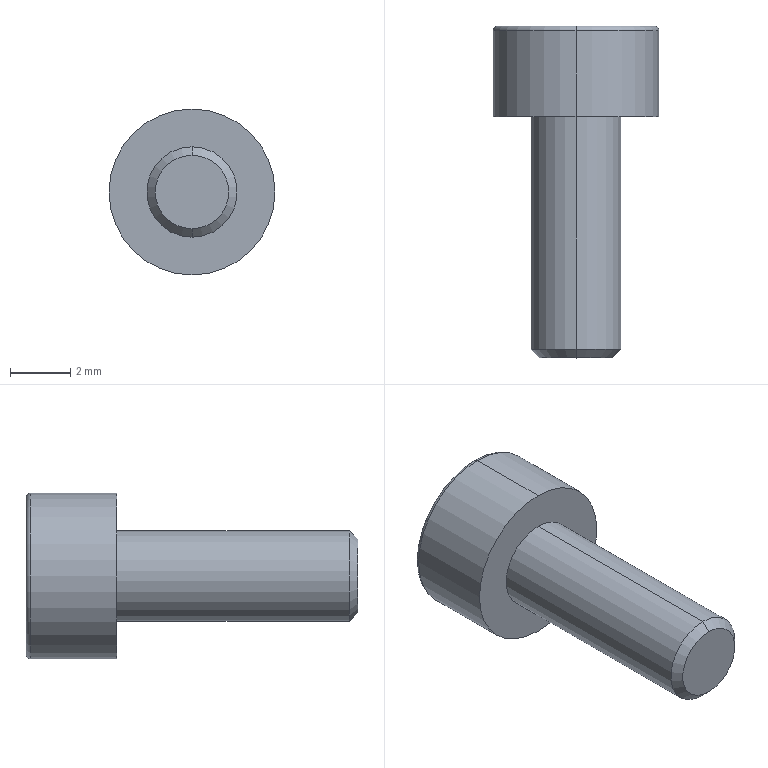Part | SolidWorks | features ICE 2, Chamfer 1, Extrusion 1, Fillet 1, RefAxis 1 | 1 solid | 18 faces | box 5.5 x 11 x 5.5 mm | volume 120.016 mm3 | plane 10 | cylinder 4 | cone 2 | torus 2 | commonest cylinder face diameters 3 x2 5.5 x2
STEP:
#1=CARTESIAN_POINT('',(0.,-8.,-1.22));
#2=VERTEX_POINT('',#1);
#3=CARTESIAN_POINT('',(0.,-8.,1.22));
#4=VERTEX_POINT('',#3);
#5=CARTESIAN_POINT('',(0.,-8.,0.));
#6=DIRECTION('',(0.,-1.,0.));
#7=DIRECTION('',(0.,0.,-1.));
#8=AXIS2_PLACEMENT_3D('',#5,#6,#7);
#9=CIRCLE('',#8,1.22);
#10=EDGE_CURVE('',#2,#4,#9,.T.);
#11=ORIENTED_EDGE('',*,*,#10,.F.);
#12=CARTESIAN_POINT('',(0.,-7.72,-1.5));
#13=VERTEX_POINT('',#12);
#14=CARTESIAN_POINT('',(0.,-8.,-1.22));
#15=DIRECTION('',(0.,0.7071,-0.7071));
#16=VECTOR('',#15,1000.);
#17=LINE('',#14,#16);
#18=EDGE_CURVE('',#2,#13,#17,.T.);
#19=ORIENTED_EDGE('',*,*,#18,.T.);
#20=CARTESIAN_POINT('',(0.,-7.72,1.5));
#21=VERTEX_POINT('',#20);
#22=CARTESIAN_POINT('',(0.,-7.72,0.));
#23=DIRECTION('',(0.,1.,0.));
#24=DIRECTION('',(0.,0.,-1.));
#25=AXIS2_PLACEMENT_3D('',#22,#23,#24);
#26=CIRCLE('',#25,1.5);
#27=EDGE_CURVE('',#21,#13,#26,.T.);
#28=ORIENTED_EDGE('',*,*,#27,.F.);
#29=CARTESIAN_POINT('',(0.,-8.,1.22));
#30=DIRECTION('',(0.,0.7071,0.7071));
#31=VECTOR('',#30,1000.);
#32=LINE('',#29,#31);
#33=EDGE_CURVE('',#4,#21,#32,.T.);
#34=ORIENTED_EDGE('',*,*,#33,.F.);
#35=EDGE_LOOP('',(#11,#19,#28,#34));
#36=FACE_OUTER_BOUND('',#35,.T.);
#37=CARTESIAN_POINT('',(0.,-8.,0.));
#38=DIRECTION('',(0.,1.,0.));
#39=DIRECTION('',(0.,0.,1.));
#40=AXIS2_PLACEMENT_3D('',#37,#38,#39);
#41=CONICAL_SURFACE('',#40,1.22,0.7854);
#42=ADVANCED_FACE('',(#36),#41,.T.);
#43=ORIENTED_EDGE('',*,*,#27,.T.);
#44=CARTESIAN_POINT('',(0.,0.,-1.5));
#45=VERTEX_POINT('',#44);
#46=CARTESIAN_POINT('',(0.,-8.,-1.5));
#47=DIRECTION('',(0.,1.,0.));
#48=VECTOR('',#47,1000.);
#49=LINE('',#46,#48);
#50=EDGE_CURVE('',#13,#45,#49,.T.);
#51=ORIENTED_EDGE('',*,*,#50,.T.);
#52=CARTESIAN_POINT('',(0.,0.,1.5));
#53=VERTEX_POINT('',#52);
#54=CARTESIAN_POINT('',(0.,0.,0.));
#55=DIRECTION('',(0.,-1.,0.));
#56=DIRECTION('',(0.,0.,1.));
#57=AXIS2_PLACEMENT_3D('',#54,#55,#56);
#58=CIRCLE('',#57,1.5);
#59=EDGE_CURVE('',#45,#53,#58,.T.);
#60=ORIENTED_EDGE('',*,*,#59,.T.);
#61=CARTESIAN_POINT('',(0.,-8.,1.5));
#62=DIRECTION('',(0.,1.,0.));
#63=VECTOR('',#62,1000.);
#64=LINE('',#61,#63);
#65=EDGE_CURVE('',#21,#53,#64,.T.);
#66=ORIENTED_EDGE('',*,*,#65,.F.);
#67=EDGE_LOOP('',(#43,#51,#60,#66));
#68=FACE_OUTER_BOUND('',#67,.T.);
#69=CARTESIAN_POINT('',(0.,-8.,0.));
#70=DIRECTION('',(0.,1.,0.));
#71=DIRECTION('',(0.,0.,1.));
#72=AXIS2_PLACEMENT_3D('',#69,#70,#71);
#73=CYLINDRICAL_SURFACE('',#72,1.5);
#74=ADVANCED_FACE('',(#68),#73,.T.);
#75=CARTESIAN_POINT('',(0.,2.85,-2.75));
#76=VERTEX_POINT('',#75);
#77=CARTESIAN_POINT('',(0.,2.85,2.75));
#78=VERTEX_POINT('',#77);
#79=CARTESIAN_POINT('',(0.,2.85,0.));
#80=DIRECTION('',(0.,-1.,0.));
#81=DIRECTION('',(0.,0.,1.));
#82=AXIS2_PLACEMENT_3D('',#79,#80,#81);
#83=CIRCLE('',#82,2.75);
#84=EDGE_CURVE('',#76,#78,#83,.T.);
#85=ORIENTED_EDGE('',*,*,#84,.F.);
#86=CARTESIAN_POINT('',(0.,3.,-2.6));
#87=VERTEX_POINT('',#86);
#88=CARTESIAN_POINT('',(0.,2.85,-2.6));
#89=DIRECTION('',(1.,0.,0.));
#90=DIRECTION('',(0.,0.,-1.));
#91=AXIS2_PLACEMENT_3D('',#88,#89,#90);
#92=CIRCLE('',#91,0.15);
#93=EDGE_CURVE('',#76,#87,#92,.T.);
#94=ORIENTED_EDGE('',*,*,#93,.T.);
#95=CARTESIAN_POINT('',(0.,3.,2.6));
#96=VERTEX_POINT('',#95);
#97=CARTESIAN_POINT('',(0.,3.,0.));
#98=DIRECTION('',(0.,1.,0.));
#99=DIRECTION('',(0.,0.,1.));
#100=AXIS2_PLACEMENT_3D('',#97,#98,#99);
#101=CIRCLE('',#100,2.6);
#102=EDGE_CURVE('',#96,#87,#101,.T.);
#103=ORIENTED_EDGE('',*,*,#102,.F.);
#104=CARTESIAN_POINT('',(0.,2.85,2.6));
#105=DIRECTION('',(-1.,0.,0.));
#106=DIRECTION('',(0.,0.,1.));
#107=AXIS2_PLACEMENT_3D('',#104,#105,#106);
#108=CIRCLE('',#107,0.15);
#109=EDGE_CURVE('',#78,#96,#108,.T.);
#110=ORIENTED_EDGE('',*,*,#109,.F.);
#111=EDGE_LOOP('',(#85,#94,#103,#110));
#112=FACE_OUTER_BOUND('',#111,.T.);
#113=CARTESIAN_POINT('',(0.,2.85,0.));
#114=DIRECTION('',(0.,1.,0.));
#115=DIRECTION('',(0.,0.,1.));
#116=AXIS2_PLACEMENT_3D('',#113,#114,#115);
#117=TOROIDAL_SURFACE('',#116,2.6,0.15);
#118=ADVANCED_FACE('',(#112),#117,.T.);
#119=ORIENTED_EDGE('',*,*,#84,.T.);
#120=CARTESIAN_POINT('',(0.,0.,2.75));
#121=VERTEX_POINT('',#120);
#122=CARTESIAN_POINT('',(0.,3.,2.75));
#123=DIRECTION('',(0.,-1.,0.));
#124=VECTOR('',#123,1000.);
#125=LINE('',#122,#124);
#126=EDGE_CURVE('',#78,#121,#125,.T.);
#127=ORIENTED_EDGE('',*,*,#126,.T.);
#128=CARTESIAN_POINT('',(0.,0.,-2.75));
#129=VERTEX_POINT('',#128);
#130=CARTESIAN_POINT('',(0.,0.,0.));
#131=DIRECTION('',(0.,1.,0.));
#132=DIRECTION('',(0.,0.,1.));
#133=AXIS2_PLACEMENT_3D('',#130,#131,#132);
#134=CIRCLE('',#133,2.75);
#135=EDGE_CURVE('',#121,#129,#134,.T.);
#136=ORIENTED_EDGE('',*,*,#135,.T.);
#137=CARTESIAN_POINT('',(0.,3.,-2.75));
#138=DIRECTION('',(0.,-1.,0.));
#139=VECTOR('',#138,1000.);
#140=LINE('',#137,#139);
#141=EDGE_CURVE('',#76,#129,#140,.T.);
#142=ORIENTED_EDGE('',*,*,#141,.F.);
#143=EDGE_LOOP('',(#119,#127,#136,#142));
#144=FACE_OUTER_BOUND('',#143,.T.);
#145=CARTESIAN_POINT('',(0.,3.,0.));
#146=DIRECTION('',(0.,-1.,0.));
#147=DIRECTION('',(0.,0.,-1.));
#148=AXIS2_PLACEMENT_3D('',#145,#146,#147);
#149=CYLINDRICAL_SURFACE('',#148,2.75);
#150=ADVANCED_FACE('',(#144),#149,.T.);
#151=CARTESIAN_POINT('',(0.,0.,0.));
#152=DIRECTION('',(0.,1.,0.));
#153=DIRECTION('',(0.,0.,1.));
#154=AXIS2_PLACEMENT_3D('',#151,#152,#153);
#155=CIRCLE('',#154,2.75);
#156=EDGE_CURVE('',#129,#121,#155,.T.);
#157=ORIENTED_EDGE('',*,*,#156,.F.);
#158=ORIENTED_EDGE('',*,*,#135,.F.);
#159=EDGE_LOOP('',(#157,#158));
#160=FACE_OUTER_BOUND('',#159,.T.);
#161=CARTESIAN_POINT('',(0.,0.,0.));
#162=DIRECTION('',(0.,-1.,0.));
#163=DIRECTION('',(0.,0.,1.));
#164=AXIS2_PLACEMENT_3D('',#161,#162,#163);
#165=CIRCLE('',#164,1.5);
#166=EDGE_CURVE('',#53,#45,#165,.T.);
#167=ORIENTED_EDGE('',*,*,#166,.F.);
#168=ORIENTED_EDGE('',*,*,#59,.F.);
#169=EDGE_LOOP('',(#167,#168));
#170=FACE_BOUND('',#169,.T.);
#171=CARTESIAN_POINT('',(0.,0.,0.));
#172=DIRECTION('',(0.,1.,0.));
#173=DIRECTION('',(0.,0.,1.));
#174=AXIS2_PLACEMENT_3D('',#171,#172,#173);
#175=PLANE('',#174);
#176=ADVANCED_FACE('',(#160,#170),#175,.F.);
#177=ORIENTED_EDGE('',*,*,#126,.F.);
#178=CARTESIAN_POINT('',(0.,2.85,0.));
#179=DIRECTION('',(0.,-1.,0.));
#180=DIRECTION('',(0.,0.,1.));
#181=AXIS2_PLACEMENT_3D('',#178,#179,#180);
#182=CIRCLE('',#181,2.75);
#183=EDGE_CURVE('',#78,#76,#182,.T.);
#184=ORIENTED_EDGE('',*,*,#183,.T.);
#185=ORIENTED_EDGE('',*,*,#141,.T.);
#186=ORIENTED_EDGE('',*,*,#156,.T.);
#187=EDGE_LOOP('',(#177,#184,#185,#186));
#188=FACE_OUTER_BOUND('',#187,.T.);
#189=CARTESIAN_POINT('',(0.,3.,0.));
#190=DIRECTION('',(0.,-1.,0.));
#191=DIRECTION('',(0.,0.,-1.));
#192=AXIS2_PLACEMENT_3D('',#189,#190,#191);
#193=CYLINDRICAL_SURFACE('',#192,2.75);
#194=ADVANCED_FACE('',(#188),#193,.T.);
#195=ORIENTED_EDGE('',*,*,#102,.T.);
#196=CARTESIAN_POINT('',(0.,3.,0.));
#197=DIRECTION('',(0.,1.,0.));
#198=DIRECTION('',(0.,0.,1.));
#199=AXIS2_PLACEMENT_3D('',#196,#197,#198);
#200=CIRCLE('',#199,2.6);
#201=EDGE_CURVE('',#87,#96,#200,.T.);
#202=ORIENTED_EDGE('',*,*,#201,.T.);
#203=EDGE_LOOP('',(#195,#202));
#204=FACE_OUTER_BOUND('',#203,.T.);
#205=CARTESIAN_POINT('',(0.739,3.,1.28));
#206=VERTEX_POINT('',#205);
#207=CARTESIAN_POINT('',(1.478,3.,0.));
#208=VERTEX_POINT('',#207);
#209=CARTESIAN_POINT('',(0.739,3.,1.28));
#210=DIRECTION('',(0.5,0.,-0.866));
#211=VECTOR('',#210,1000.);
#212=LINE('',#209,#211);
#213=EDGE_CURVE('',#206,#208,#212,.T.);
#214=ORIENTED_EDGE('',*,*,#213,.F.);
#215=CARTESIAN_POINT('',(-0.739,3.,1.28));
#216=VERTEX_POINT('',#215);
#217=CARTESIAN_POINT('',(-0.739,3.,1.28));
#218=DIRECTION('',(1.,0.,0.));
#219=VECTOR('',#218,1000.);
#220=LINE('',#217,#219);
#221=EDGE_CURVE('',#216,#206,#220,.T.);
#222=ORIENTED_EDGE('',*,*,#221,.F.);
#223=CARTESIAN_POINT('',(-1.478,3.,0.));
#224=VERTEX_POINT('',#223);
#225=CARTESIAN_POINT('',(-1.478,3.,0.));
#226=DIRECTION('',(0.5,0.,0.866));
#227=VECTOR('',#226,1000.);
#228=LINE('',#225,#227);
#229=EDGE_CURVE('',#224,#216,#228,.T.);
#230=ORIENTED_EDGE('',*,*,#229,.F.);
#231=CARTESIAN_POINT('',(-0.739,3.,-1.28));
#232=VERTEX_POINT('',#231);
#233=CARTESIAN_POINT('',(-0.739,3.,-1.28));
#234=DIRECTION('',(-0.5,0.,0.866));
#235=VECTOR('',#234,1000.);
#236=LINE('',#233,#235);
#237=EDGE_CURVE('',#232,#224,#236,.T.);
#238=ORIENTED_EDGE('',*,*,#237,.F.);
#239=CARTESIAN_POINT('',(0.739,3.,-1.28));
#240=VERTEX_POINT('',#239);
#241=CARTESIAN_POINT('',(0.739,3.,-1.28));
#242=DIRECTION('',(-1.,0.,0.));
#243=VECTOR('',#242,1000.);
#244=LINE('',#241,#243);
#245=EDGE_CURVE('',#240,#232,#244,.T.);
#246=ORIENTED_EDGE('',*,*,#245,.F.);
#247=CARTESIAN_POINT('',(1.478,3.,0.));
#248=DIRECTION('',(-0.5,0.,-0.866));
#249=VECTOR('',#248,1000.);
#250=LINE('',#247,#249);
#251=EDGE_CURVE('',#208,#240,#250,.T.);
#252=ORIENTED_EDGE('',*,*,#251,.F.);
#253=EDGE_LOOP('',(#214,#222,#230,#238,#246,#252));
#254=FACE_BOUND('',#253,.T.);
#255=CARTESIAN_POINT('',(0.,3.,0.));
#256=DIRECTION('',(0.,1.,0.));
#257=DIRECTION('',(0.,0.,1.));
#258=AXIS2_PLACEMENT_3D('',#255,#256,#257);
#259=PLANE('',#258);
#260=ADVANCED_FACE('',(#204,#254),#259,.T.);
#261=ORIENTED_EDGE('',*,*,#213,.T.);
#262=CARTESIAN_POINT('',(1.478,1.7,0.));
#263=VERTEX_POINT('',#262);
#264=CARTESIAN_POINT('',(1.478,1.7,0.));
#265=DIRECTION('',(0.,1.,0.));
#266=VECTOR('',#265,1000.);
#267=LINE('',#264,#266);
#268=EDGE_CURVE('',#263,#208,#267,.T.);
#269=ORIENTED_EDGE('',*,*,#268,.F.);
#270=CARTESIAN_POINT('',(0.739,1.7,1.28));
#271=VERTEX_POINT('',#270);
#272=CARTESIAN_POINT('',(0.739,1.7,1.28));
#273=DIRECTION('',(0.5,0.,-0.866));
#274=VECTOR('',#273,1000.);
#275=LINE('',#272,#274);
#276=EDGE_CURVE('',#271,#263,#275,.T.);
#277=ORIENTED_EDGE('',*,*,#276,.F.);
#278=CARTESIAN_POINT('',(0.739,1.7,1.28));
#279=DIRECTION('',(0.,1.,0.));
#280=VECTOR('',#279,1000.);
#281=LINE('',#278,#280);
#282=EDGE_CURVE('',#271,#206,#281,.T.);
#283=ORIENTED_EDGE('',*,*,#282,.T.);
#284=EDGE_LOOP('',(#261,#269,#277,#283));
#285=FACE_OUTER_BOUND('',#284,.T.);
#286=CARTESIAN_POINT('',(0.739,1.7,1.28));
#287=DIRECTION('',(0.866,0.,0.5));
#288=DIRECTION('',(0.5,0.,-0.866));
#289=AXIS2_PLACEMENT_3D('',#286,#287,#288);
#290=PLANE('',#289);
#291=ADVANCED_FACE('',(#285),#290,.F.);
#292=ORIENTED_EDGE('',*,*,#221,.T.);
#293=ORIENTED_EDGE('',*,*,#282,.F.);
#294=CARTESIAN_POINT('',(-0.739,1.7,1.28));
#295=VERTEX_POINT('',#294);
#296=CARTESIAN_POINT('',(-0.739,1.7,1.28));
#297=DIRECTION('',(1.,0.,0.));
#298=VECTOR('',#297,1000.);
#299=LINE('',#296,#298);
#300=EDGE_CURVE('',#295,#271,#299,.T.);
#301=ORIENTED_EDGE('',*,*,#300,.F.);
#302=CARTESIAN_POINT('',(-0.739,1.7,1.28));
#303=DIRECTION('',(0.,1.,0.));
#304=VECTOR('',#303,1000.);
#305=LINE('',#302,#304);
#306=EDGE_CURVE('',#295,#216,#305,.T.);
#307=ORIENTED_EDGE('',*,*,#306,.T.);
#308=EDGE_LOOP('',(#292,#293,#301,#307));
#309=FACE_OUTER_BOUND('',#308,.T.);
#310=CARTESIAN_POINT('',(-0.739,1.7,1.28));
#311=DIRECTION('',(0.,0.,1.));
#312=DIRECTION('',(1.,0.,0.));
#313=AXIS2_PLACEMENT_3D('',#310,#311,#312);
#314=PLANE('',#313);
#315=ADVANCED_FACE('',(#309),#314,.F.);
#316=ORIENTED_EDGE('',*,*,#229,.T.);
#317=ORIENTED_EDGE('',*,*,#306,.F.);
#318=CARTESIAN_POINT('',(-1.478,1.7,0.));
#319=VERTEX_POINT('',#318);
#320=CARTESIAN_POINT('',(-1.478,1.7,0.));
#321=DIRECTION('',(0.5,0.,0.866));
#322=VECTOR('',#321,1000.);
#323=LINE('',#320,#322);
#324=EDGE_CURVE('',#319,#295,#323,.T.);
#325=ORIENTED_EDGE('',*,*,#324,.F.);
#326=CARTESIAN_POINT('',(-1.478,1.7,0.));
#327=DIRECTION('',(0.,1.,0.));
#328=VECTOR('',#327,1000.);
#329=LINE('',#326,#328);
#330=EDGE_CURVE('',#319,#224,#329,.T.);
#331=ORIENTED_EDGE('',*,*,#330,.T.);
#332=EDGE_LOOP('',(#316,#317,#325,#331));
#333=FACE_OUTER_BOUND('',#332,.T.);
#334=CARTESIAN_POINT('',(-1.478,1.7,0.));
#335=DIRECTION('',(-0.866,0.,0.5));
#336=DIRECTION('',(0.5,0.,0.866));
#337=AXIS2_PLACEMENT_3D('',#334,#335,#336);
#338=PLANE('',#337);
#339=ADVANCED_FACE('',(#333),#338,.F.);
#340=ORIENTED_EDGE('',*,*,#237,.T.);
#341=ORIENTED_EDGE('',*,*,#330,.F.);
#342=CARTESIAN_POINT('',(-0.739,1.7,-1.28));
#343=VERTEX_POINT('',#342);
#344=CARTESIAN_POINT('',(-0.739,1.7,-1.28));
#345=DIRECTION('',(-0.5,0.,0.866));
#346=VECTOR('',#345,1000.);
#347=LINE('',#344,#346);
#348=EDGE_CURVE('',#343,#319,#347,.T.);
#349=ORIENTED_EDGE('',*,*,#348,.F.);
#350=CARTESIAN_POINT('',(-0.739,1.7,-1.28));
#351=DIRECTION('',(0.,1.,0.));
#352=VECTOR('',#351,1000.);
#353=LINE('',#350,#352);
#354=EDGE_CURVE('',#343,#232,#353,.T.);
#355=ORIENTED_EDGE('',*,*,#354,.T.);
#356=EDGE_LOOP('',(#340,#341,#349,#355));
#357=FACE_OUTER_BOUND('',#356,.T.);
#358=CARTESIAN_POINT('',(-0.739,1.7,-1.28));
#359=DIRECTION('',(-0.866,0.,-0.5));
#360=DIRECTION('',(-0.5,0.,0.866));
#361=AXIS2_PLACEMENT_3D('',#358,#359,#360);
#362=PLANE('',#361);
#363=ADVANCED_FACE('',(#357),#362,.F.);
#364=ORIENTED_EDGE('',*,*,#245,.T.);
#365=ORIENTED_EDGE('',*,*,#354,.F.);
#366=CARTESIAN_POINT('',(0.739,1.7,-1.28));
#367=VERTEX_POINT('',#366);
#368=CARTESIAN_POINT('',(0.739,1.7,-1.28));
#369=DIRECTION('',(-1.,0.,0.));
#370=VECTOR('',#369,1000.);
#371=LINE('',#368,#370);
#372=EDGE_CURVE('',#367,#343,#371,.T.);
#373=ORIENTED_EDGE('',*,*,#372,.F.);
#374=CARTESIAN_POINT('',(0.739,1.7,-1.28));
#375=DIRECTION('',(0.,1.,0.));
#376=VECTOR('',#375,1000.);
#377=LINE('',#374,#376);
#378=EDGE_CURVE('',#367,#240,#377,.T.);
#379=ORIENTED_EDGE('',*,*,#378,.T.);
#380=EDGE_LOOP('',(#364,#365,#373,#379));
#381=FACE_OUTER_BOUND('',#380,.T.);
#382=CARTESIAN_POINT('',(0.739,1.7,-1.28));
#383=DIRECTION('',(0.,0.,-1.));
#384=DIRECTION('',(-1.,0.,0.));
#385=AXIS2_PLACEMENT_3D('',#382,#383,#384);
#386=PLANE('',#385);
#387=ADVANCED_FACE('',(#381),#386,.F.);
#388=ORIENTED_EDGE('',*,*,#251,.T.);
#389=ORIENTED_EDGE('',*,*,#378,.F.);
#390=CARTESIAN_POINT('',(1.478,1.7,0.));
#391=DIRECTION('',(-0.5,0.,-0.866));
#392=VECTOR('',#391,1000.);
#393=LINE('',#390,#392);
#394=EDGE_CURVE('',#263,#367,#393,.T.);
#395=ORIENTED_EDGE('',*,*,#394,.F.);
#396=ORIENTED_EDGE('',*,*,#268,.T.);
#397=EDGE_LOOP('',(#388,#389,#395,#396));
#398=FACE_OUTER_BOUND('',#397,.T.);
#399=CARTESIAN_POINT('',(1.478,1.7,0.));
#400=DIRECTION('',(0.866,0.,-0.5));
#401=DIRECTION('',(-0.5,0.,-0.866));
#402=AXIS2_PLACEMENT_3D('',#399,#400,#401);
#403=PLANE('',#402);
#404=ADVANCED_FACE('',(#398),#403,.F.);
#405=ORIENTED_EDGE('',*,*,#276,.T.);
#406=ORIENTED_EDGE('',*,*,#394,.T.);
#407=ORIENTED_EDGE('',*,*,#372,.T.);
#408=ORIENTED_EDGE('',*,*,#348,.T.);
#409=ORIENTED_EDGE('',*,*,#324,.T.);
#410=ORIENTED_EDGE('',*,*,#300,.T.);
#411=EDGE_LOOP('',(#405,#406,#407,#408,#409,#410));
#412=FACE_OUTER_BOUND('',#411,.T.);
#413=CARTESIAN_POINT('',(0.,1.7,0.));
#414=DIRECTION('',(0.,1.,0.));
#415=DIRECTION('',(0.,0.,1.));
#416=AXIS2_PLACEMENT_3D('',#413,#414,#415);
#417=PLANE('',#416);
#418=ADVANCED_FACE('',(#412),#417,.T.);
#419=ORIENTED_EDGE('',*,*,#93,.F.);
#420=ORIENTED_EDGE('',*,*,#183,.F.);
#421=ORIENTED_EDGE('',*,*,#109,.T.);
#422=ORIENTED_EDGE('',*,*,#201,.F.);
#423=EDGE_LOOP('',(#419,#420,#421,#422));
#424=FACE_OUTER_BOUND('',#423,.T.);
#425=CARTESIAN_POINT('',(0.,2.85,0.));
#426=DIRECTION('',(0.,1.,0.));
#427=DIRECTION('',(0.,0.,1.));
#428=AXIS2_PLACEMENT_3D('',#425,#426,#427);
#429=TOROIDAL_SURFACE('',#428,2.6,0.15);
#430=ADVANCED_FACE('',(#424),#429,.T.);
#431=ORIENTED_EDGE('',*,*,#50,.F.);
#432=CARTESIAN_POINT('',(0.,-7.72,0.));
#433=DIRECTION('',(0.,1.,0.));
#434=DIRECTION('',(0.,0.,-1.));
#435=AXIS2_PLACEMENT_3D('',#432,#433,#434);
#436=CIRCLE('',#435,1.5);
#437=EDGE_CURVE('',#13,#21,#436,.T.);
#438=ORIENTED_EDGE('',*,*,#437,.T.);
#439=ORIENTED_EDGE('',*,*,#65,.T.);
#440=ORIENTED_EDGE('',*,*,#166,.T.);
#441=EDGE_LOOP('',(#431,#438,#439,#440));
#442=FACE_OUTER_BOUND('',#441,.T.);
#443=CARTESIAN_POINT('',(0.,-8.,0.));
#444=DIRECTION('',(0.,1.,0.));
#445=DIRECTION('',(0.,0.,1.));
#446=AXIS2_PLACEMENT_3D('',#443,#444,#445);
#447=CYLINDRICAL_SURFACE('',#446,1.5);
#448=ADVANCED_FACE('',(#442),#447,.T.);
#449=CARTESIAN_POINT('',(0.,-8.,0.));
#450=DIRECTION('',(0.,-1.,0.));
#451=DIRECTION('',(0.,0.,-1.));
#452=AXIS2_PLACEMENT_3D('',#449,#450,#451);
#453=CIRCLE('',#452,1.22);
#454=EDGE_CURVE('',#4,#2,#453,.T.);
#455=ORIENTED_EDGE('',*,*,#454,.T.);
#456=ORIENTED_EDGE('',*,*,#10,.T.);
#457=EDGE_LOOP('',(#455,#456));
#458=FACE_OUTER_BOUND('',#457,.T.);
#459=CARTESIAN_POINT('',(0.,-8.,0.));
#460=DIRECTION('',(0.,-1.,0.));
#461=DIRECTION('',(0.,0.,-1.));
#462=AXIS2_PLACEMENT_3D('',#459,#460,#461);
#463=PLANE('',#462);
#464=ADVANCED_FACE('',(#458),#463,.T.);
#465=ORIENTED_EDGE('',*,*,#18,.F.);
#466=ORIENTED_EDGE('',*,*,#454,.F.);
#467=ORIENTED_EDGE('',*,*,#33,.T.);
#468=ORIENTED_EDGE('',*,*,#437,.F.);
#469=EDGE_LOOP('',(#465,#466,#467,#468));
#470=FACE_OUTER_BOUND('',#469,.T.);
#471=CARTESIAN_POINT('',(0.,-8.,0.));
#472=DIRECTION('',(0.,1.,0.));
#473=DIRECTION('',(0.,0.,1.));
#474=AXIS2_PLACEMENT_3D('',#471,#472,#473);
#475=CONICAL_SURFACE('',#474,1.22,0.7854);
#476=ADVANCED_FACE('',(#470),#475,.T.);
#477=CLOSED_SHELL('',(#42,#74,#118,#150,#176,#194,#260,#291,#315,#339,#363,#387,#404,#418,#430,#448,#464,#476));
#478=MANIFOLD_SOLID_BREP('',#477);
#479=CARTESIAN_POINT('',(0.,0.,0.));
#480=DIRECTION('',(0.,0.,1.));
#481=DIRECTION('',(1.,0.,0.));
#482=AXIS2_PLACEMENT_3D('',#479,#480,#481);
#483=(LENGTH_UNIT()NAMED_UNIT(*)SI_UNIT(.MILLI.,.METRE.));
#484=UNCERTAINTY_MEASURE_WITH_UNIT(LENGTH_MEASURE(0.00001),#483,'','');
#485=(NAMED_UNIT(*)PLANE_ANGLE_UNIT()SI_UNIT($,.RADIAN.));
#486=(NAMED_UNIT(*)SI_UNIT($,.STERADIAN.)SOLID_ANGLE_UNIT());
#487=(GEOMETRIC_REPRESENTATION_CONTEXT(3)GLOBAL_UNCERTAINTY_ASSIGNED_CONTEXT((#484))GLOBAL_UNIT_ASSIGNED_CONTEXT((#483,#485,#486))REPRESENTATION_CONTEXT('',''));
#488=ADVANCED_BREP_SHAPE_REPRESENTATION('',(#478,#482),#487);